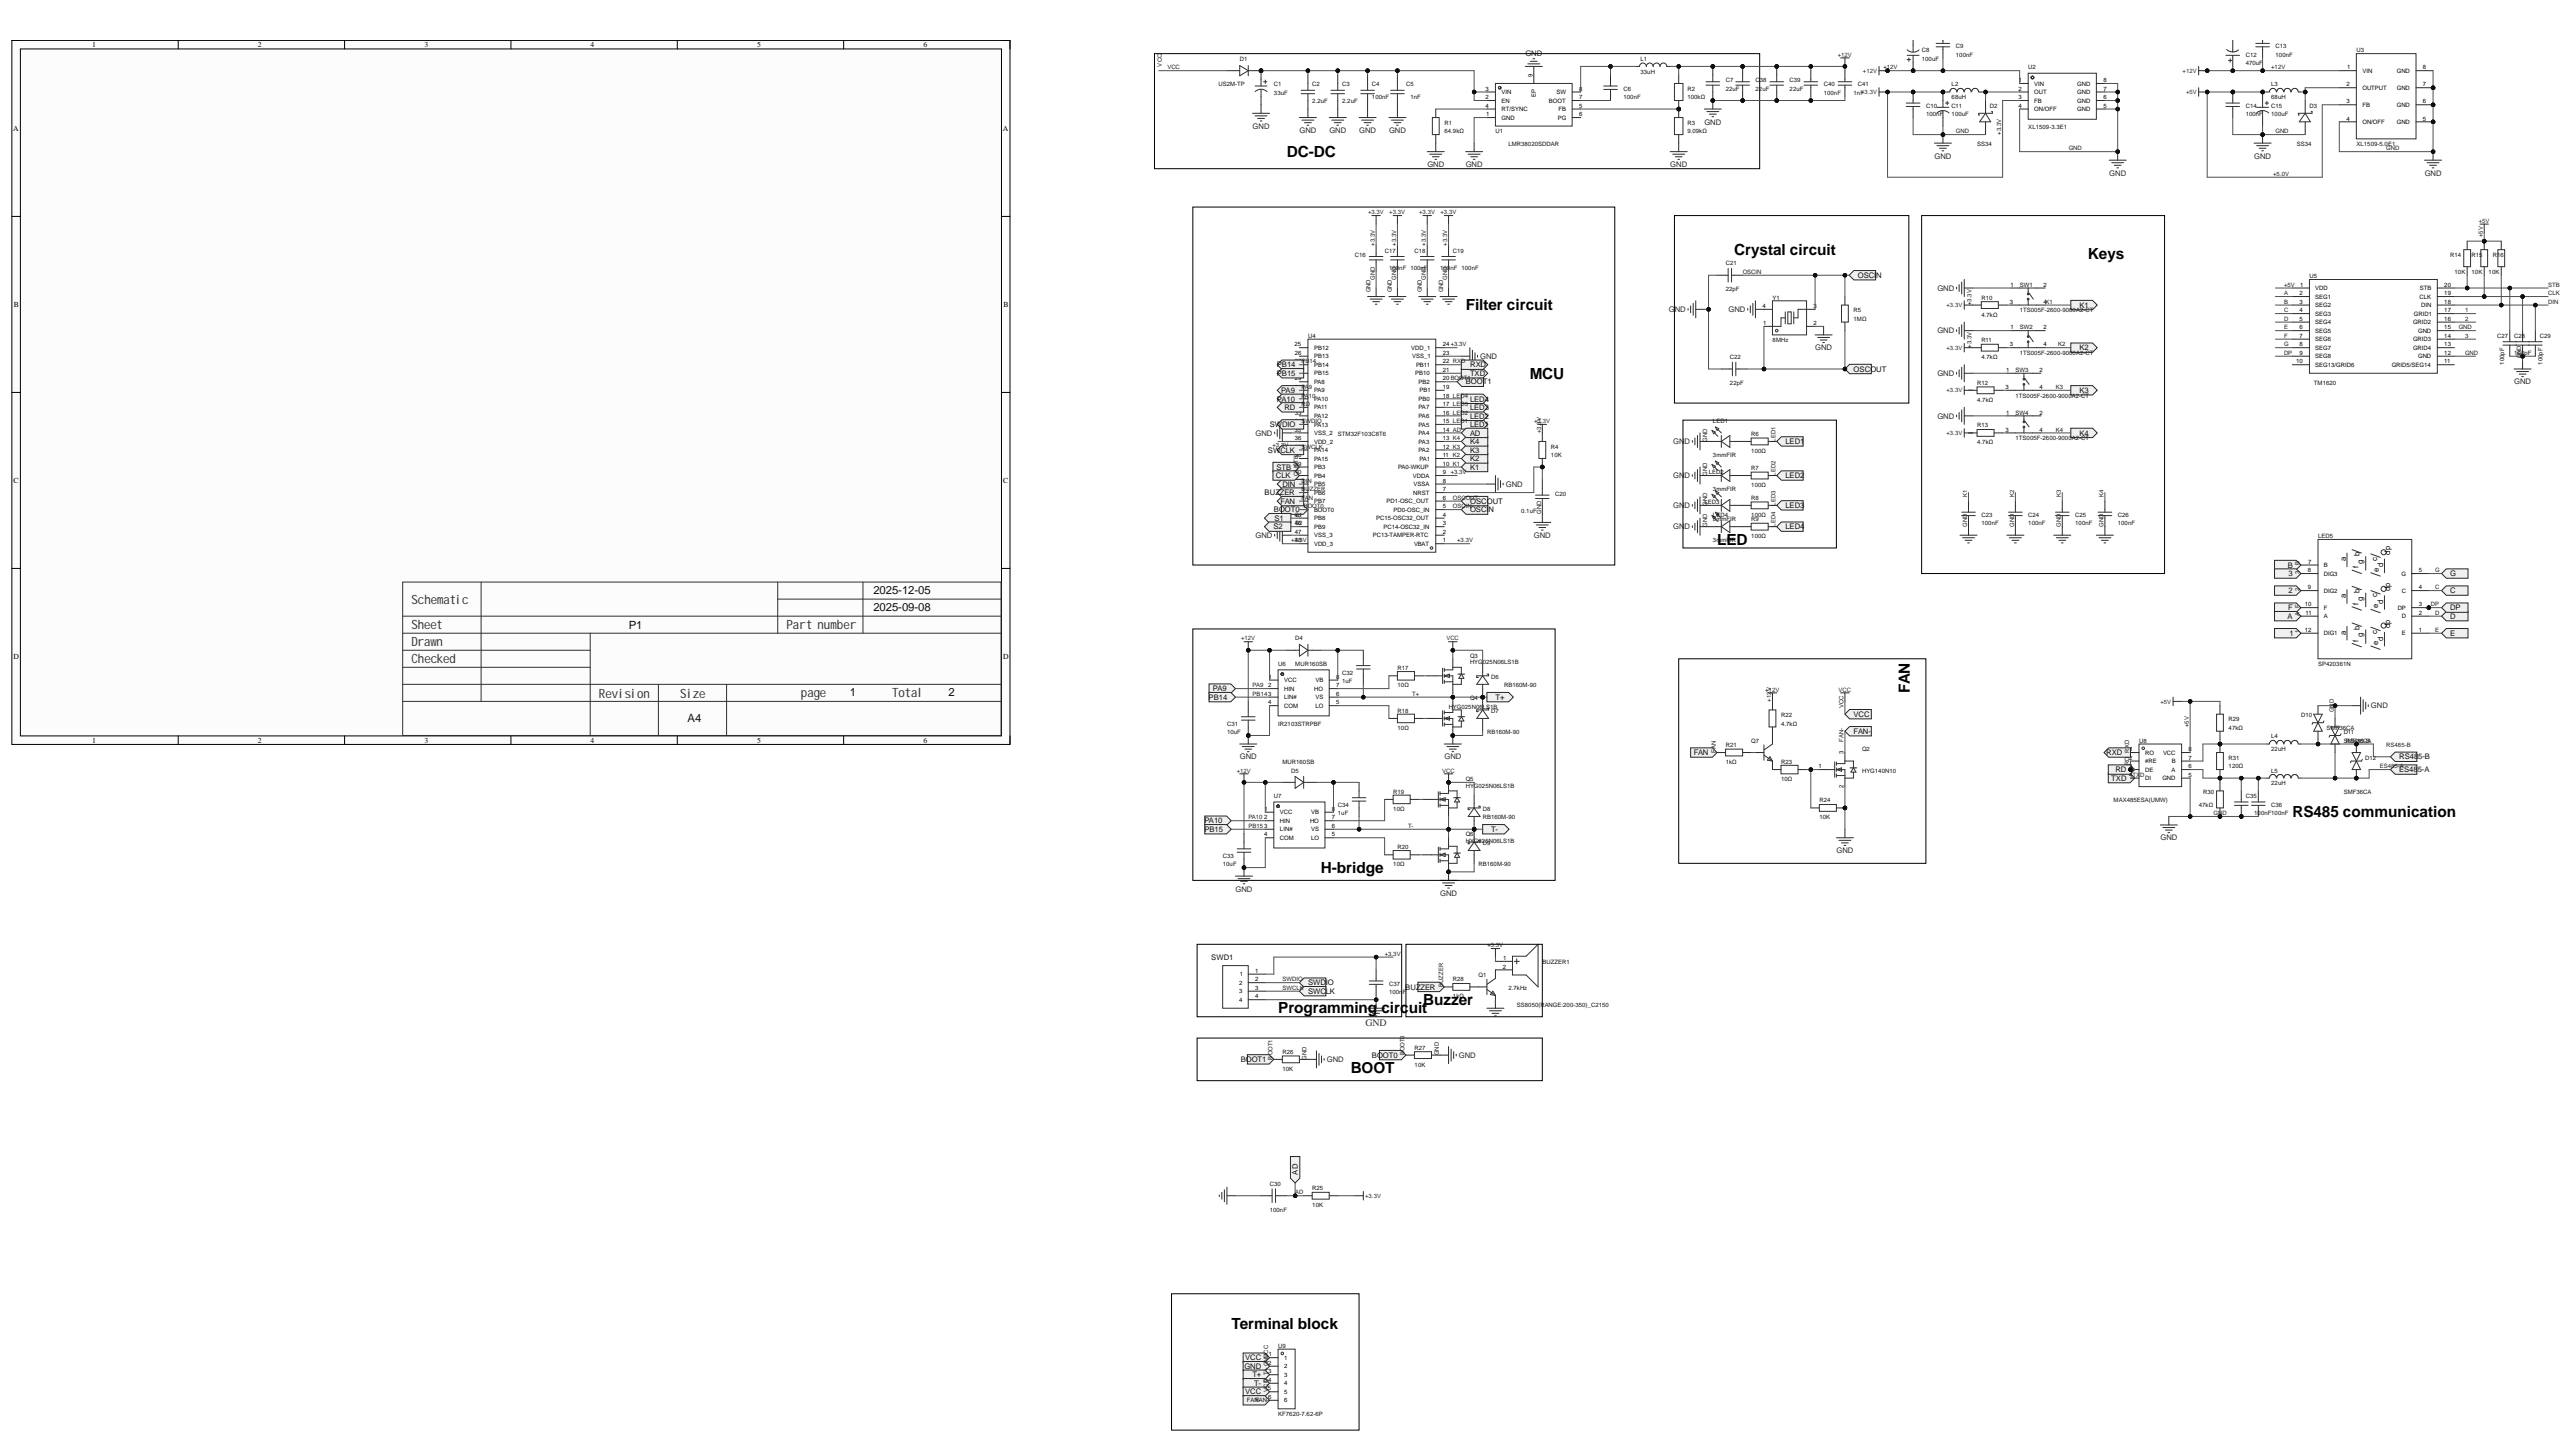Circuit board | Altium Designer | 117 parts | 82 nets
Bill of materials:
Comment,Description,Designator,Footprint,LibRef,Quantity
"2.7kHz","Driving method: active (built-in driver circuit); frequency: 2.7kHz; sound pressure (SPL): 80dB;","BUZZER1","BUZ-SMD_L9.6-W9.6-LS10.0-R","YS-SBZ9650DYB05","1"
"33uF","Capacitance: 33uF; tolerance: ±20%; rated voltage: 100V; ripple current: -; equivalent series resistance (ESR): -;","C1","CAP-TH_BD8.0-P3.50-D1.0-FD","ECF1KM330F12OTPO","1"
"2.2uF","Capacitance: 2.2uF; tolerance: ±10%; rated voltage: 100V; dielectric (temperature coefficient): X8L;","C2, C3","C1206","GRM31CL8EL225KE07L","2"
"100nF","","C4","C1206","CAP_1206","1"
"1nF","","C5","C1206","CAP_1206","1"
"100nF","Capacitance: 100nF; tolerance: ±10%; rated voltage: 50V; temperature coefficient: X7R;","C6, C9, C10, C13, C14, C16, C17, C18, C19, C23, C24, C25, C26, C30, C35, C36, C37, C40","C0805","CL21B104KBCNNNC","18"
"22uF","Capacitance: 22uF; tolerance: ±10%; rated voltage: 25V; dielectric (temperature coefficient): X7S;","C7, C38, C39","C1210","GRJ32EC71E226KE11L","3"
"100uF","Capacitance: 100uF; tolerance: ±20%; rated voltage: 25V; ripple current: 54mA@120Hz;","C8, C11, C15","CAP-SMD_BD6.3-L6.6-W6.6-LS7.3-FD_JVS25V100M6X4","JVS25V100M6X4","3"
"470uF","Capacitance: 470uF; tolerance: ±20%; rated voltage: 35V; ripple current: 525mA@120Hz; equivalent series resistance: -;","C12","CAP-TH_BD10.0-P5.00-D1.0-FD","35PX470MEFC10X12.5","1"
"0.1uF","","C20","C0805","CAP_0805","1"
"22pF","Capacitance: 22pF; tolerance: ±5%; rated voltage: 50V; temperature coefficient: C0G;","C21, C22","C0805","CL21C220JBANNNC","2"
"100pF","Capacitance: 100pF; tolerance: ±5%; rated voltage: 50V; temperature coefficient: C0G;","C27, C28, C29","C0805","CL21C101JBANNNC","3"
"10uF","Capacitance: 10uF; tolerance: ±10%; rated voltage: 50V; temperature coefficient: X5R;","C31, C33","C0805","0805X5R106K500NT","2"
"1uF","Capacitance: 10uF; tolerance: ±10%; rated voltage: 50V; temperature coefficient: X5R;","C32, C34","C0805","0805X5R106K500NT","2"
"1nF","Capacitance: 1nF; tolerance: ±10%; rated voltage: 50V; temperature coefficient: X7R;","C41","C0805","CL21B102KBCNNNC","1"
"US2M-TP","Diode configuration: -; forward voltage (Vf): 1.7V@2A; DC reverse voltage (Vr): 1kV; rectified current: 2A; reverse recovery time (Trr): 100ns;","D1","SMB_L4.6-W3.6-LS5.3-RD","US2M-TP","1"
"SS34","Diode configuration: single; forward voltage (Vf): 550mV@3A; DC reverse voltage (Vr): 40V; rectified current: 3A;","D2, D3","SMA_L4.3-W2.6-LS5.2-RD","SS34_C8678","2"
"MUR160SB","Diode configuration: single; forward voltage (Vf): 1.3V@1A; DC reverse voltage (Vr): 600V; rectified current: 1A; reverse recovery time (Trr): 50ns;","D4, D5","SMB_L4.6-W3.6-LS5.3-RD","MUR160SB","2"
"RB160M-90","Forward voltage (Vf): 750mV@1.0A; DC reverse voltage (Vr): 90V; rectified current: 1A;","D6, D7, D8, D9","SOD-123FL_L2.7-W1.8-LS3.7-RD","RB160M-90","4"
"SMF36CA","Polarity: bidirectional; reverse standoff voltage (Vrwm): 36V; clamping voltage: 58.1V; peak pulse current (Ipp): 3.5A; peak pulse power (Ppp): 200W@10/1000us; breakdown voltage: 40V;","D10, D11, D12","SOD-123_L2.7-W1.8-LS3.7-BI","SMF36CA_C435502","3"
"33uH","Inductance: 33uH; tolerance: ±20%; rated current: 4.4A; saturation current (Isat): 5A; type: molded inductor;","L1","IND-SMD_L11.5-W10.0_FXL1040","FXL1040-330-M","1"
"68uH","Inductance: 68uH; tolerance: ±20%; rated current: 1.5A; saturation current (Isat): 2A; type: -;","L2, L3","IND-SMD_L7.1-W6.6_H5.0","PSPMAA0605H-680M-IGF","2"
"22uH","Inductance: 22uH; tolerance: ±10%; rated current: 5mA; saturation current (Isat): -; DC resistance (DCR): 900mΩ;","L4, L5","L1206","SCL3216T220KSP","2"
"3mmFIR","","LED1, LED2, LED3, LED4","LED-TH_BD3.0-P2.54-FD","3mmFIR","4"
"SP420361N","Number of digits: 3; character size (inch): 0.36; color: red; LED polarity: common cathode;","LED5","LED-SEG-TH_SP420361N","SP420361N","1"
"SS8050(RANGE:200-350)","Transistor type: NPN; collector current (Ic): 1.5A; collector-emitter breakdown voltage (Vceo): 25V; power (Pd): 300mW; DC current gain (hFE@Ic,Vce): 200@800mA,1V;","Q1, Q7","SOT-23-3_L2.9-W1.3-P1.90-LS2.4-BR","SS8050(RANGE:200-350)_C2150","2"
"HYG140N10","Type: 1 N-channel; drain-source voltage (Vdss): 100V; continuous drain current (Id): 45A; on-resistance (RDS(on)@Vgs,Id): -; power (Pd): 3W; threshold voltage (Vgs(th)@Id): 2.5V@250uA;","Q2","TO-252-3_L6.6-W6.1-P4.58-LS10.1-BR","NCE0140K2-VB","1"
"HYG025N06LS1B","Quantity: 1 N-channel; drain-source voltage (Vdss): 60V; continuous drain current (Id): 160A; on-resistance (RDS(on)): 3.3mΩ@10V; power dissipation (Pd): 125W; threshold voltage (Vgs(th)): 3V@250uA;","Q3, Q4, Q5, Q6","TO-263-2_L10.2-W8.7-P5.08-LS15.1-BR","HYG025N06LS1B","4"
"64.9kΩ","Resistor type: thick film resistor; resistance: 64.9kΩ; tolerance: ±1%; power: 125mW; operating voltage: 150V; temperature coefficient: ±100ppm/?;","R1","R0805","CR0805-FX-6492ELF","1"
"100kΩ","Resistor type: thick film resistor; resistance: 100kΩ; tolerance: ±5%; power: 100mW; temperature coefficient: ±200ppm/?;","R2","R0805","CR0805-10W-104JT","1"
"9.09kΩ","Resistance: 24.9kΩ; tolerance: ±1%; power: 125mW;","R3","R0805","RCA0524K9FLF","1"
"10K","","R4, R14, R15, R16, R24, R25, R26, R27","R0805","Res_0805","8"
"1MΩ","Resistor type: thick film resistor; resistance: 1MΩ; tolerance: ±1%; power: 125mW; max operating voltage: 150V; temperature coefficient: ±100ppm/?;","R5","R0805","0805W8F1004T5E","1"
"100Ω","Resistor type: thick film resistor; resistance: 100Ω; tolerance: ±1%; power: 125mW; max operating voltage: 150V; temperature coefficient: ±100ppm/?;","R6, R7, R8, R9","R0805","0805W8F1000T5E","4"
"4.7kΩ","Resistor type: thick film resistor; resistance: 4.7kΩ; tolerance: ±5%; power: 125mW; operating voltage: 150V; temperature coefficient: ±100ppm/?;, Resistor type: thick film resistor; resistance: 4.7kΩ; tolerance: ±1%; power: 125mW; max operating voltage: 150V; temperature coefficient: ±100ppm/?;","R10, R11, R12, R13, R22","R0805","0805W8J0472T5E, 0805W8F4701T5E","5"
"10Ω","Resistor type: thick film resistor; resistance: 10Ω; tolerance: ±1%; power: 125mW; temperature coefficient: ±100ppm/?;","R17, R18, R19, R20, R23","R0805","CRCW080510R0FKEAC","5"
"1kΩ","Resistor type: thick film resistor; resistance: 1kΩ; tolerance: ±1%; power: 125mW; max operating voltage: 150V; temperature coefficient: ±100ppm/?;","R21, R28","R0805","0805W8F1001T5E","2"
"47kΩ","Resistor type: thick film resistor; resistance: 47kΩ; tolerance: ±1%; power: 125mW; operating voltage: 150V; temperature coefficient: ±100ppm/?;","R29, R30","R0805","0805W8F4702T5E","2"
"120Ω","Resistor type: thick film resistor; resistance: 120Ω; tolerance: ±1%; power: 125mW; max operating voltage: 150V; temperature coefficient: ±100ppm/?;","R31","R0805","0805W8F1200T5E","1"
"1TS005F-2600-9000A2-CT","6*6*9mm 立贴 260克力不锈钢覆银弹片轻触开关","SW1, SW2, SW3, SW4","SW-SMD_4P-L6.0-W6.0-P4.50-LS9.0-2","1TS005F-2600-9000A2-CT","4"
"220S-1*4P H=8.5MM Ytype Gold-plated","","SWD1","DIP-1X4P2.54","220S-1*4P H=8.5MM Ytype Gold-plated","1"
"LMR38020SDDAR","Function type: buck; output type: adjustable; input voltage: 4.2V~80V; output voltage: 1V~75V; output current: 2A;","U1","ESOP-8_L4.9-W3.9-P1.27-LS6.0-BL-EP-1","LMR38020SDDAR","1"
"XL1509-3.3E1","Function type: buck; operating voltage: 4.5V~40V; output voltage: 3.3V; output current: 2A; output type: fixed;","U2","SOP-8_L4.9-W3.9-P1.27-LS6.0-BL","XL1509-3.3E1","1"
"XL1509-5.0E1","Function type: buck; operating voltage: 4.5V~40V; output voltage: 5V; output current: 2A; output type: fixed;","U3","SOIC-8_L5.0-W4.0-P1.27-LS6.0-BL","XL1509-5.0E1","1"
"STM32F103C8T6","CPU core: ARM-M3; max CPU frequency: 72MHz; application field: -;","U4","LQFP-48_L7.0-W7.0-P0.50-LS9.0-BL","STM32F103C8T6","1"
"TM1620","显示模式（8段×6位~10段x4位）的LED 驱动IC","U5","SOIC-20_L13.0-W7.6-P1.27-LS10.3-BL","TM1620","1"
"IR2103STRPBF","Driver configuration: half-bridge; load type: IGBT; MOSFET; driver channels: 2; sink current (IOL): 270mA; source current (IOH): 130mA; operating voltage: 10V~20V; rise time (tr): 100ns; fall time (tf): 50ns;","U6","SOIC-8_L4.9-W3.9-P1.27-LS6.0-BL","IR2103STRPBF","1"
"","Driver configuration: half-bridge; load type: IGBT; MOSFET; driver channels: 2; sink current (IOL): 270mA; source current (IOH): 130mA; operating voltage: 10V~20V; rise time (tr): 100ns; fall time (tf): 50ns;","U7","SOIC-8_L4.9-W3.9-P1.27-LS6.0-BL","IR2103STRPBF","1"
"MAX485ESA(UMW)","","U8","SOP-8_L5.0-W4.0-P1.27-LS6.0-BL","MAX485ESA(UMW)","1"
"KF7620-7.62-6P","","U9","CONN-TH_6P-P7.62_KF7620-7.62-6P","KF7620-7.62-6P","1"
"8MHz","Crystal type: SMD crystal; frequency: 8MHz; frequency tolerance at room temperature: ±10ppm; load capacitance: 20pF; frequency stability: ±20ppm;","Y1","CRYSTAL-SMD_4P-L3.2-W2.5-BL","XL2SI-111-8M","1"
Netlist (Protel format):
[
BUZZER1
BUZ-SMD_L9.6-W9.6-LS10.0-R
2.7kHz



]
[
C1
CAP-TH_BD8.0-P3.50-D1.0-FD
33uF



]
[
C2
C1206
2.2uF



]
[
C3
C1206
2.2uF



]
[
C4
C1206
100nF



]
[
C5
C1206
1nF



]
[
C6
C0805
100nF



]
[
C7
C1210
22uF



]
[
C8
CAP-SMD_BD6.3-L6.6-W6.6-LS7.3-FD_JVS25V100M6X4
100uF



]
[
C9
C0805
100nF



]
[
C10
C0805
100nF



]
[
C11
CAP-SMD_BD6.3-L6.6-W6.6-LS7.3-FD_JVS25V100M6X4
100uF



]
[
C12
CAP-TH_BD10.0-P5.00-D1.0-FD
470uF



]
[
C13
C0805
100nF



]
[
C14
C0805
100nF



]
[
C15
CAP-SMD_BD6.3-L6.6-W6.6-LS7.3-FD_JVS25V100M6X4
100uF



]
[
C16
C0805
100nF



]
[
C17
C0805
100nF



]
[
C18
C0805
100nF



]
[
C19
C0805
100nF



]
[
C20
C0805
0.1uF



]
[
C21
C0805
22pF



]
[
C22
C0805
22pF



]
[
C23
C0805
100nF



]
[
C24
C0805
100nF



]
[
C25
C0805
100nF



]
[
C26
C0805
100nF



]
[
C27
C0805
100pF



]
[
C28
C0805
100pF



]
[
C29
C0805
100pF



]
[
C30
C0805
100nF



]
[
C31
C0805
10uF



]
[
C32
C0805
1uF



]
[
C33
C0805
10uF



]
[
C34
C0805
1uF



]
[
C35
C0805
100nF



]
[
C36
C0805
100nF



]
[
C37
C0805
100nF



]
[
C38
C1210
22uF



]
[
C39
C1210
22uF



]
[
C40
C0805
100nF



]
[
C41
C0805
1nF



]
[
D1
SMB_L4.6-W3.6-LS5.3-RD
US2M-TP



]
[
D2
SMA_L4.3-W2.6-LS5.2-RD
SS34



]
[
D3
SMA_L4.3-W2.6-LS5.2-RD
SS34



]
[
D4
SMB_L4.6-W3.6-LS5.3-RD
MUR160SB



]
[
D5
SMB_L4.6-W3.6-LS5.3-RD
MUR160SB



]
[
D6
SOD-123FL_L2.7-W1.8-LS3.7-RD
RB160M-90



]
[
D7
SOD-123FL_L2.7-W1.8-LS3.7-RD
RB160M-90



]
[
D8
SOD-123FL_L2.7-W1.8-LS3.7-RD
RB160M-90



]
[
D9
SOD-123FL_L2.7-W1.8-LS3.7-RD
RB160M-90



]
[
D10
SOD-123_L2.7-W1.8-LS3.7-BI
SMF36CA



]
[
D11
SOD-123_L2.7-W1.8-LS3.7-BI
SMF36CA



]
[
D12
SOD-123_L2.7-W1.8-LS3.7-BI
SMF36CA



]
[
L1
IND-SMD_L11.5-W10.0_FXL1040
33uH



]
[
L2
IND-SMD_L7.1-W6.6_H5.0
68uH



]
[
L3
IND-SMD_L7.1-W6.6_H5.0
68uH



]
[
L4
L1206
22uH



]
[
L5
L1206
22uH



]
[
LED1
LED-TH_BD3.0-P2.54-FD
3mmFIR



]
[
LED2
LED-TH_BD3.0-P2.54-FD
3mmFIR



]
[
LED3
LED-TH_BD3.0-P2.54-FD
3mmFIR



]
[
LED4
LED-TH_BD3.0-P2.54-FD
3mmFIR



]
[
LED5
LED-SEG-TH_SP420361N
SP420361N



]
[
Q1
SOT-23-3_L2.9-W1.3-P1.90-LS2.4-BR
SS8050(RANGE:200-350)



]
[
Q2
TO-252-3_L6.6-W6.1-P4.58-LS10.1-BR
HYG140N10



]
[
Q3
TO-263-2_L10.2-W8.7-P5.08-LS15.1-BR
HYG025N06LS1B



]
[
Q4
TO-263-2_L10.2-W8.7-P5.08-LS15.1-BR
HYG025N06LS1B



]
[
Q5
TO-263-2_L10.2-W8.7-P5.08-LS15.1-BR
HYG025N06LS1B



]
[
Q6
TO-263-2_L10.2-W8.7-P5.08-LS15.1-BR
HYG025N06LS1B



]
[
Q7
SOT-23-3_L2.9-W1.3-P1.90-LS2.4-BR
SS8050(RANGE:200-350)



]
[
R1
R0805
64.9kΩ



]
[
R2
R0805
100kΩ



]
[
R3
R0805
9.09kΩ



]
[
R4
R0805
10K



]
[
R5
R0805
1MΩ



]
[
R6
R0805
100Ω



]
[
R7
R0805
100Ω



]
[
R8
R0805
100Ω



]
[
R9
R0805
100Ω



]
[
R10
R0805
4.7kΩ



]
[
R11
R0805
4.7kΩ



]
[
R12
R0805
4.7kΩ



]
[
R13
R0805
4.7kΩ



]
[
R14
R0805
10K



]
[
R15
R0805
10K



]
[
R16
R0805
10K



]
[
R17
R0805
10Ω



]
[
R18
R0805
10Ω



]
[
R19
R0805
10Ω



]
[
R20
R0805
10Ω



]
[
R21
R0805
1kΩ



]
[
R22
R0805
4.7kΩ



]
[
R23
R0805
10Ω



]
[
R24
R0805
10K



]
[
R25
R0805
10K



]
[
R26
R0805
10K



]
[
R27
R0805
10K



]
[
R28
R0805
1kΩ



]
[
R29
R0805
47kΩ



]
[
R30
R0805
47kΩ



]
[
R31
R0805
120Ω



]
[
SW1
SW-SMD_4P-L6.0-W6.0-P4.50-LS9.0-2
1TS005F-2600-9000A2-CT



]
[
SW2
SW-SMD_4P-L6.0-W6.0-P4.50-LS9.0-2
1TS005F-2600-9000A2-CT



]
[
SW3
SW-SMD_4P-L6.0-W6.0-P4.50-LS9.0-2
1TS005F-2600-9000A2-CT



]
[
SW4
SW-SMD_4P-L6.0-W6.0-P4.50-LS9.0-2
1TS005F-2600-9000A2-CT



]
[
SWD1
DIP-1X4P2.54
220S-1*4P H=8.5MM Ytype Gold-plated



]
[
U1
ESOP-8_L4.9-W3.9-P1.27-LS6.0-BL-EP-1
LMR38020SDDAR



]
[
U2
SOP-8_L4.9-W3.9-P1.27-LS6.0-BL
XL1509-3.3E1



]
[
U3
SOIC-8_L5.0-W4.0-P1.27-LS6.0-BL
XL1509-5.0E1



]
[
U4
LQFP-48_L7.0-W7.0-P0.50-LS9.0-BL
STM32F103C8T6



]
[
U5
SOIC-20_L13.0-W7.6-P1.27-LS10.3-BL
TM1620



]
[
U6
SOIC-8_L4.9-W3.9-P1.27-LS6.0-BL
IR2103STRPBF



]
[
U7
SOIC-8_L4.9-W3.9-P1.27-LS6.0-BL




]
[
U8
SOP-8_L5.0-W4.0-P1.27-LS6.0-BL
MAX485ESA(UMW)



]
[
U9
CONN-TH_6P-P7.62_KF7620-7.62-6P
KF7620-7.62-6P



]
[
Y1
CRYSTAL-SMD_4P-L3.2-W2.5-BL
8MHz



]
(
VCC
D1-2
D6-1
D8-1
Q3-4
Q5-4
U9-1
U9-5
)
(
TXD
U4-21
U8-4
)
(
T-
C34-1
D8-2
D9-1
Q5-3
Q6-4
U7-6
U9-4
)
(
T+
C32-1
D6-2
D7-1
Q3-3
Q4-4
U6-6
U9-3
)
(
SWDIO
SWD1-2
U4-34
)
(
SWCLK
SWD1-3
U4-37
)
(
STB
C27-1
R14-1
U4-39
U5-20
)
(
RXD
U4-22
U8-1
)
(
RS485-B
D10-1
D12-2
L4-2
)
(
RD
U4-32
U8-2
U8-3
)
(
PB15
U4-28
U7-3
)
(
PB14
U4-27
U6-3
)
(
PA10
U4-31
U7-2
)
(
PA9
U4-30
U6-2
)
(
OSCOUT
C22-1
R5-1
U4-6
Y1-1
)
(
OSCIN
C21-1
R5-2
U4-5
Y1-3
)
(
NetR20_1
R20-1
U7-5
)
(
NetR19_1
R19-1
U7-7
)
(
NetR18_1
R18-1
U6-5
)
(
NetR17_1
R17-1
U6-7
)
(
NetR13_2
R13-2
SW4-3
)
(
NetR12_2
R12-2
SW3-3
)
(
NetR11_2
R11-2
SW2-3
)
(
NetR10_2
R10-2
SW1-3
)
(
NetR2_1
R2-1
R3-2
U1-5
)
(
NetR1_2
R1-2
U1-4
)
(
NetQ7_3
Q7-3
R22-1
)
(
NetQ7_2
Q7-2
R23-1
)
(
NetQ7_1
Q7-1
R21-2
)
(
NetQ6_1
Q6-1
R20-2
)
(
NetQ5_1
Q5-1
R19-2
)
(
NetQ4_1
Q4-1
R18-2
)
(
NetQ3_1
Q3-1
R17-2
)
(
NetQ2_1
Q2-1
R23-2
R24-1
)
(
NetQ1_1
Q1-1
R28-2
)
(
NetLED4_1
LED4-1
R9-1
)
(
NetLED3_1
LED3-1
R8-1
)
(
NetLED2_1
LED2-1
R7-1
)
(
NetLED1_1
LED1-1
R6-1
)
(
NetL4_1
L4-1
R29-1
R31-2
U8-7
)
(
NetD3_1
D3-1
L3-2
U3-2
)
(
NetD2_1
D2-1
L2-2
U2-2
)
(
NetC35_2
C35-2
C36-1
L5-1
R30-2
R31-1
U8-6
)
(
NetC34_2
C34-2
D5-1
U7-8
)
(
NetC32_2
C32-2
D4-1
U6-8
)
(
NetC20_2
C20-2
R4-1
U4-7
)
(
NetC6_2
C6-2
L1-1
U1-8
)
(
NetC6_1
C6-1
U1-7
)
(
NetC1_1
C1-1
C2-2
C3-2
C4-2
C5-2
D1-1
U1-2
U1-3
)
(
NetBUZZER1_2
BUZZER1-2
Q1-3
)
(
LED4
R9-2
U4-18
)
(
LED3
R8-2
U4-17
)
(
LED2
R7-2
U4-16
)
(
LED1
R6-2
U4-15
)
(
K4
C26-2
SW4-4
U4-13
)
(
K3
C25-2
SW3-4
U4-12
)
(
K2
C24-2
SW2-4
U4-11
)
(
K1
C23-2
SW1-4
U4-10
)
(
GND
C1-2
C2-1
C3-1
C4-1
C5-1
C7-1
C8-2
C9-2
C10-1
C11-2
C12-2
C13-2
C14-1
C15-2
C16-1
C17-1
C18-1
C19-1
C20-1
C21-2
C22-2
C23-1
C24-1
C25-1
C26-1
C27-2
C28-2
C29-1
C30-2
C31-1
C33-1
C35-1
C36-2
C37-1
C38-1
C39-1
C40-1
C41-1
D2-2
D3-2
D7-2
D9-2
D10-2
D11-2
LED1-2
LED2-2
LED3-2
LED4-2
Q1-2
Q2-2
Q4-3
Q6-3
R1-1
R3-1
R24-2
R26-2
R27-2
R30-1
SW1-1
SW2-1
SW3-1
SW4-1
SWD1-4
U1-1
U1-9
U2-4
U2-5
U2-6
U2-7
U2-8
U3-4
U3-5
U3-6
U3-7
U3-8
U4-8
U4-23
U4-35
U4-47
U5-12
U5-15
U6-4
U7-4
U8-5
U9-2
Y1-2
Y1-4
)
(
G
LED5-5
U5-8
)
(
FAN-
Q2-3
U9-6
)
(
FAN
R21-1
U4-43
)
(
F
LED5-10
U5-7
)
(
ES485-A
D11-1
D12-1
L5-2
)
(
E
LED5-1
U5-6
)
(
DP
LED5-3
U5-9
)
(
DIN
C29-2
R16-1
U4-41
U5-18
)
(
D
LED5-2
U5-5
)
(
CLK
C28-1
R15-1
U4-40
U5-19
)
(
C
LED5-4
U5-4
)
(
BUZZER
R28-1
U4-42
)
(
BOOT1
R26-1
U4-20
)
(
BOOT0
R27-1
U4-44
)
(
B
LED5-7
U5-3
)
(
AD
C30-1
R25-1
U4-14
)
(
A
LED5-11
U5-2
)
(
+12V
C7-2
C8-1
C9-1
C12-1
C13-1
C31-2
C33-2
C38-2
C39-2
C40-2
C41-2
D4-2
D5-2
L1-2
R2-2
R22-2
U2-1
U3-1
U6-1
U7-1
)
(
+5.0V
C14-2
C15-1
L3-1
R14-2
R15-2
R16-2
R29-2
U3-3
U5-1
U8-8
)
(
+3.3V
BUZZER1-1
C10-2
C11-1
C16-2
C17-2
C18-2
C19-2
C37-2
L2-1
R4-2
R10-1
R11-1
R12-1
R13-1
R25-2
SWD1-1
U2-3
U4-1
U4-9
U4-24
U4-36
U4-48
)
(
3
LED5-8
U5-14
)
(
2
LED5-9
U5-16
)
(
1
LED5-12
U5-17
)